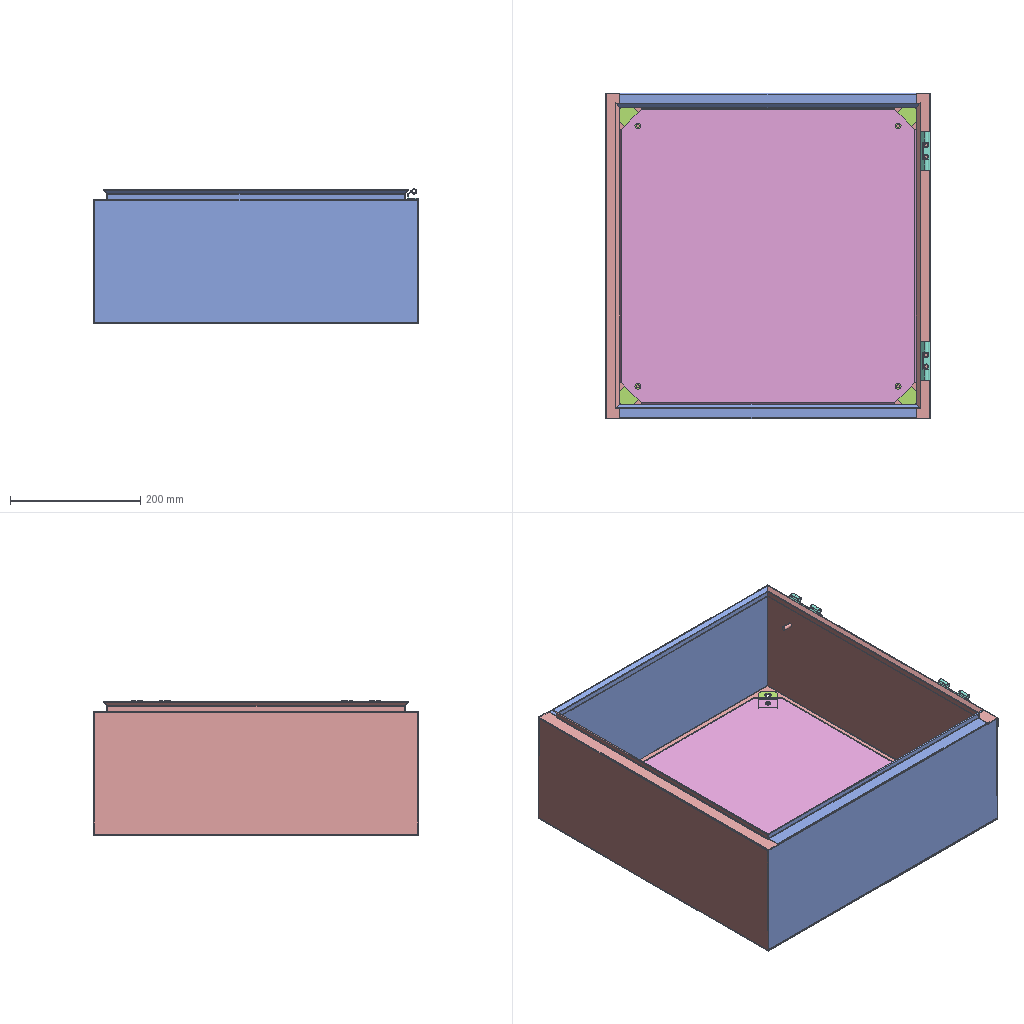Assembly | SolidWorks | 6 different items | 11 placed | box 500 x 500 x 207 mm
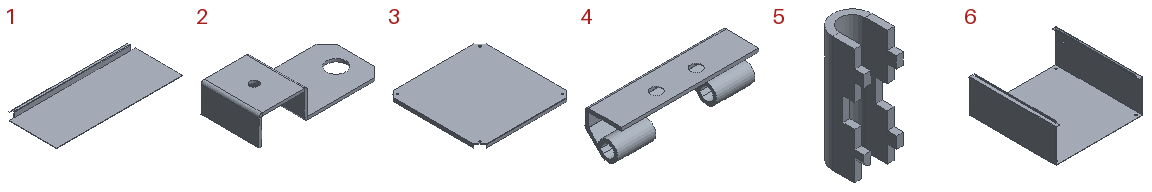Parts list (item | quantity | size | volume | features):
1 | x2 | 496.5 x 203.157 x 22 mm | 165083 mm3 | features EdgeFlange 3, SMBaseFlange 2, FlatPattern 1, SheetMetal 1
2 | x4 | 65 x 30 x 15 mm | 3912 mm3 | features EdgeFlange 2, ICE 2, Chamfer 1, FlatPattern 1, SMBaseFlange 1, SheetMetal 1
3 | x1 | 454 x 454 x 16 mm | 449338 mm3 | features EdgeFlange 2, LPattern 2, Chamfer 1, FlatPattern 1, ICE 1, SMBaseFlange 1, SheetMetal 1
4 | x2 | 60 x 16 x 16.21 mm | 3571 mm3 | features EdgeFlange 2, ICE 2, Chamfer 1, FlatPattern 1, Hem 1, LPattern 1, SMBaseFlange 1, SheetMetal 1
5 | x1 | 8.5 x 11 x 25 mm | 759.819 mm3 | features Fillet 1, FlatPattern 1, ICE 1, SMBaseFlange 1, SheetMetal 1
6 | x1 | 500 x 500 x 205.157 mm | 710210 mm3 | features EdgeFlange 6, LPattern 4, ICE 3, SMBaseFlange 3, FlatPattern 1, SheetMetal 1
Mates (type | each side: item.copy, entity, surface, feature):
Coincident | 6.1 face plane Edge-Flange1 | 1.1 face plane Base-Flange1
DistanceDim | 6.1 face plane Edge-Flange2 | 1.1 face plane Edge-Flange1
DistanceDim | 6.1 face plane Edge-Flange1 | 1.1 face plane Base-Flange1
Concentric | 6.1 face cylinder LPattern2 | 2.1 face cylinder Cut-Extrude1
Coincident | 6.1 face plane Base-Flange1 | 2.1 face plane Edge-Flange2
PlanarAngleDim | 6.1 face plane Edge-Flange1 | 2.1 face plane Edge-Flange1
Coincident | 2.1 face plane Base-Flange1 | 2.2 face plane Base-Flange1
Concentric | 6.1 face cylinder LPattern1 | 2.2 face cylinder Cut-Extrude1
PlanarAngleDim | 6.1 face plane Edge-Flange1 | 2.2 face plane Base-Flange1
Coincident | 2.1 face plane Base-Flange1 | 2.3 face plane Base-Flange1
Concentric | 6.1 face cylinder LPattern2 | 2.3 face cylinder Cut-Extrude1
Coincident | 2.4 face plane Base-Flange1 | 2.3 face plane Base-Flange1
Concentric | 6.1 face cylinder Cut-Extrude1 | 2.4 face cylinder Cut-Extrude1
PlanarAngleDim | 2.4 face plane Edge-Flange1 | 6.1 face plane Edge-Flange1
DistanceDim | 3.1 face plane Edge-Flange1 | 6.1 face plane Edge-Flange1
DistanceDim | 6.1 face plane Base-Flange1 | 3.1 face plane Edge-Flange2
Coincident | 6.1 face plane Edge-Flange2 | 4.1 face plane Base-Flange1
Concentric | 6.1 face cylinder Cut-Extrude2 | 4.1 edge
Concentric | 6.1 face cylinder LPattern3 | 4.1 edge
Coincident | 4.2 face plane Base-Flange1 | 4.1 face plane Base-Flange1
Concentric | 6.1 face cylinder LPattern4 | 4.2 edge | 2 times
Coincident | 6.1 face plane Edge-Flange2 | 1.2 face plane Edge-Flange1 | 2 times
Coincident | 6.1 face plane Edge-Flange1 | 1.2 face plane Base-Flange1